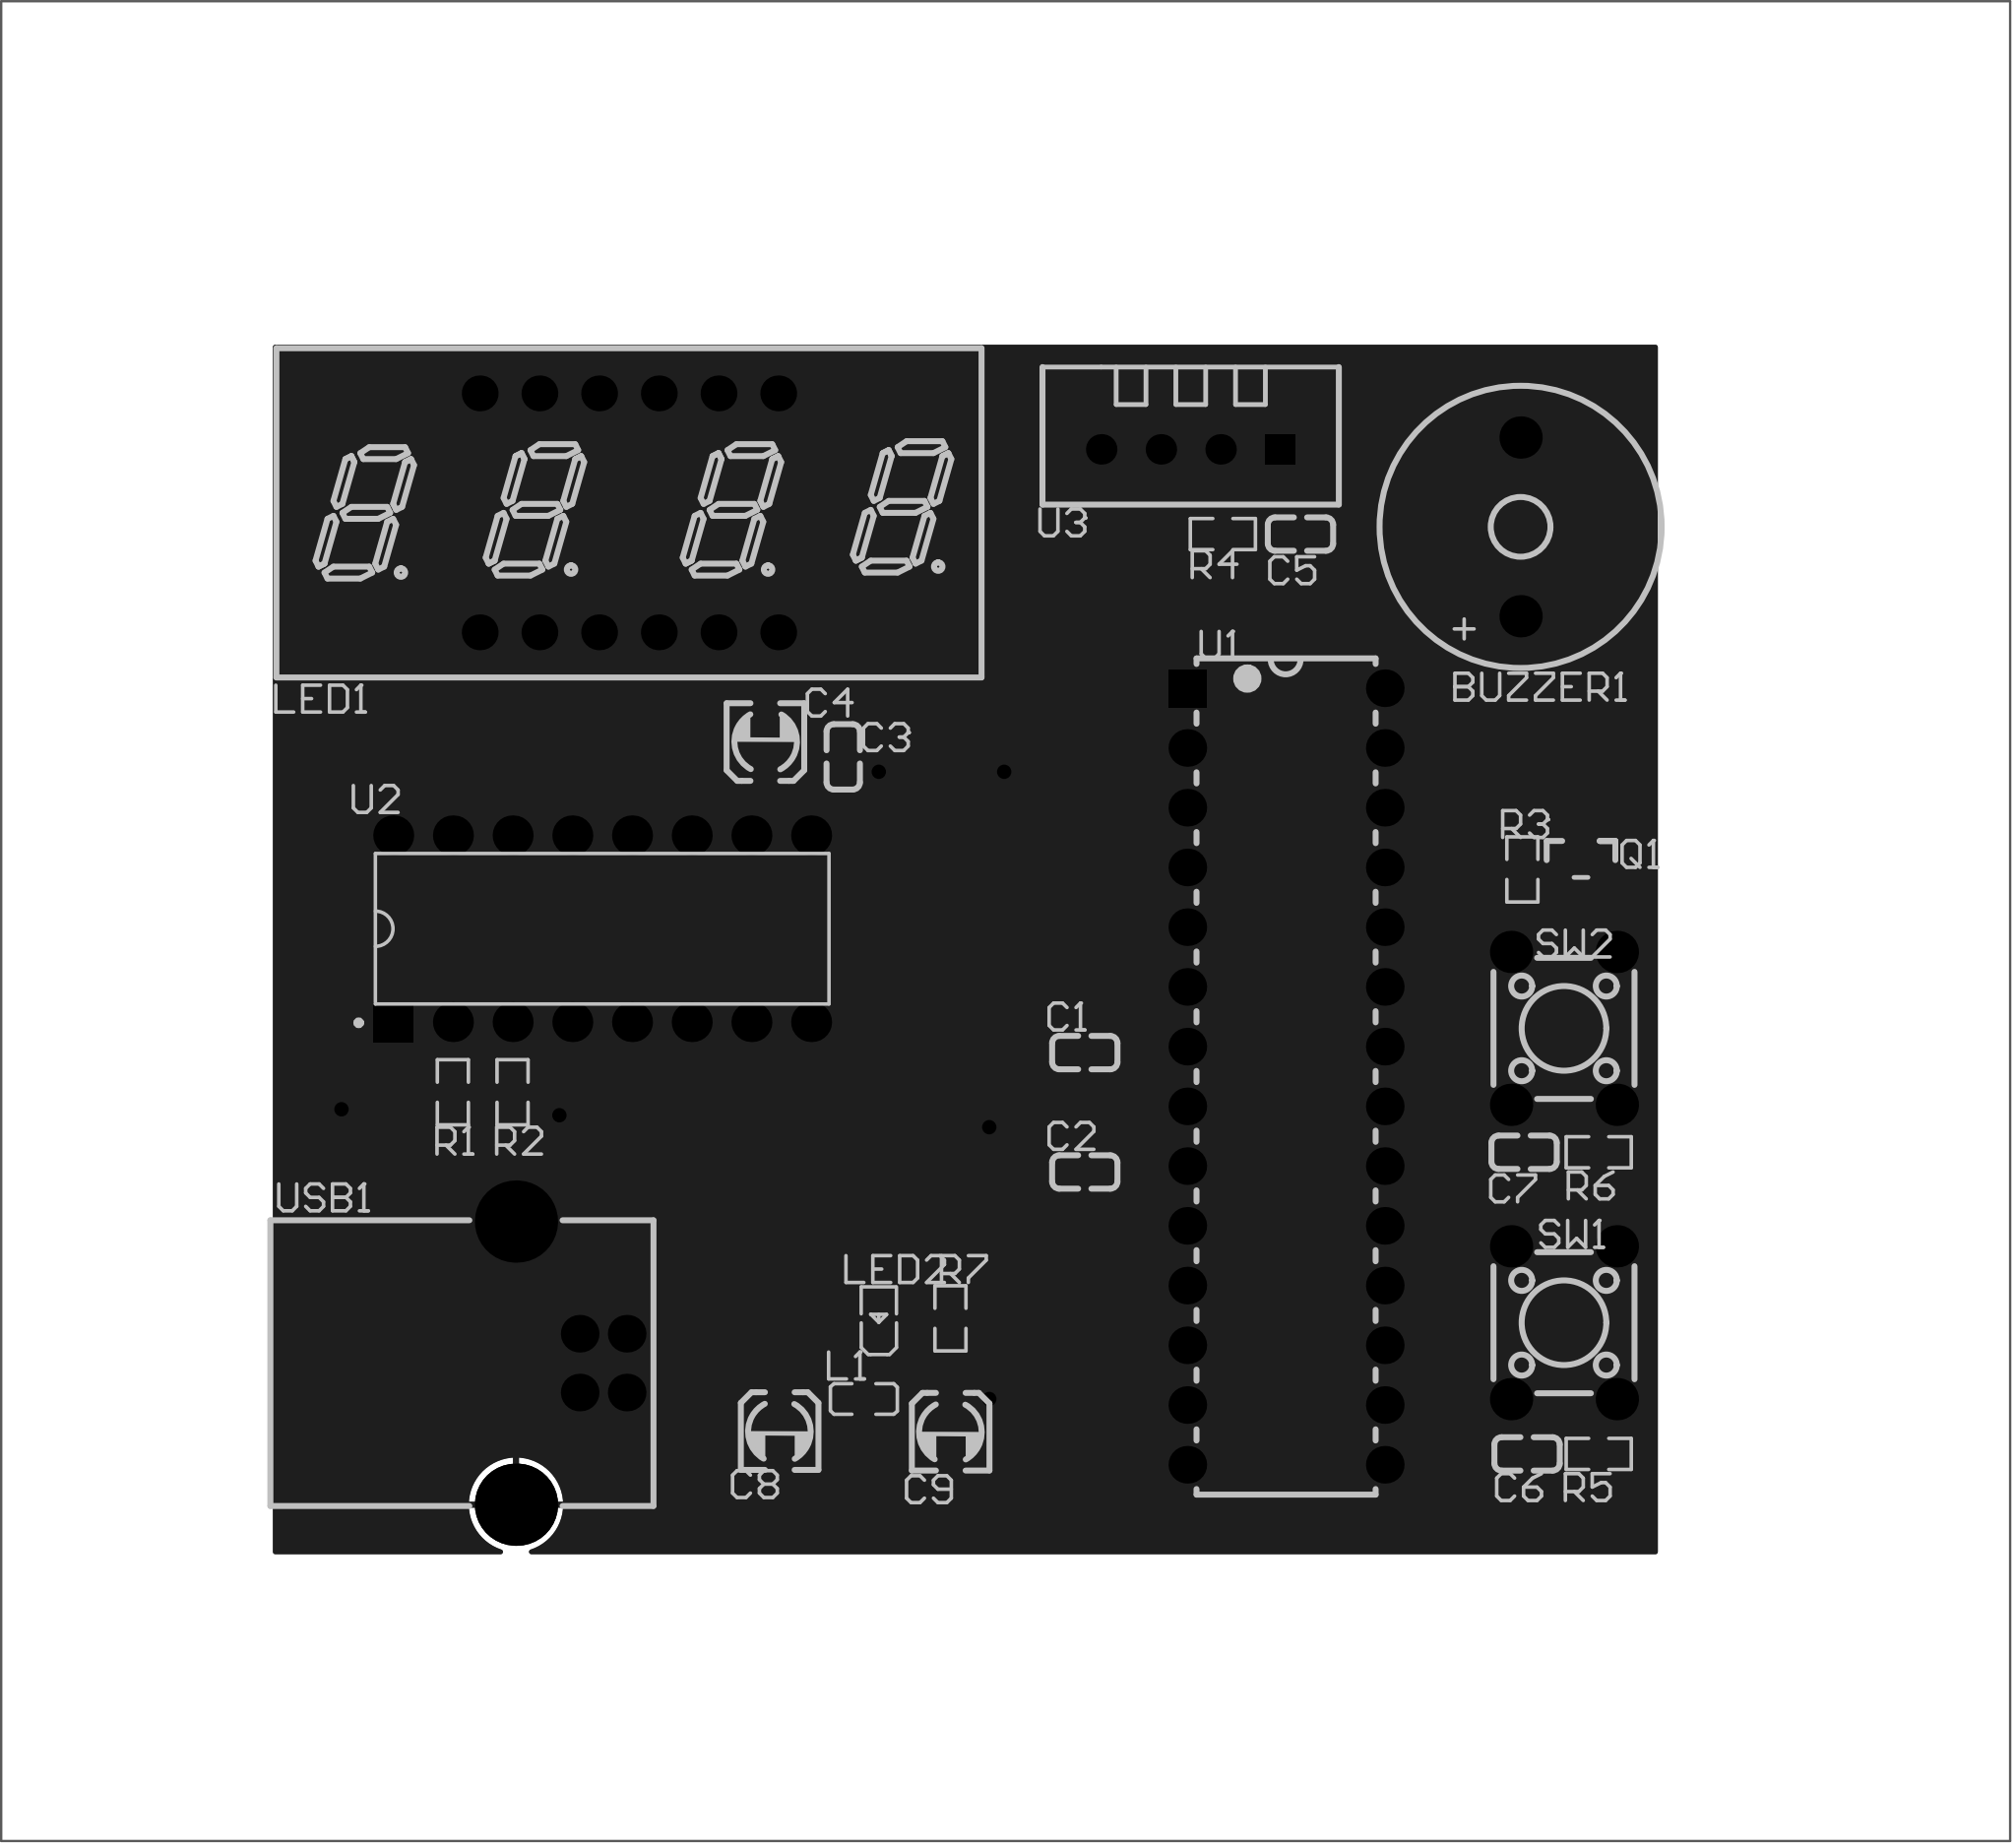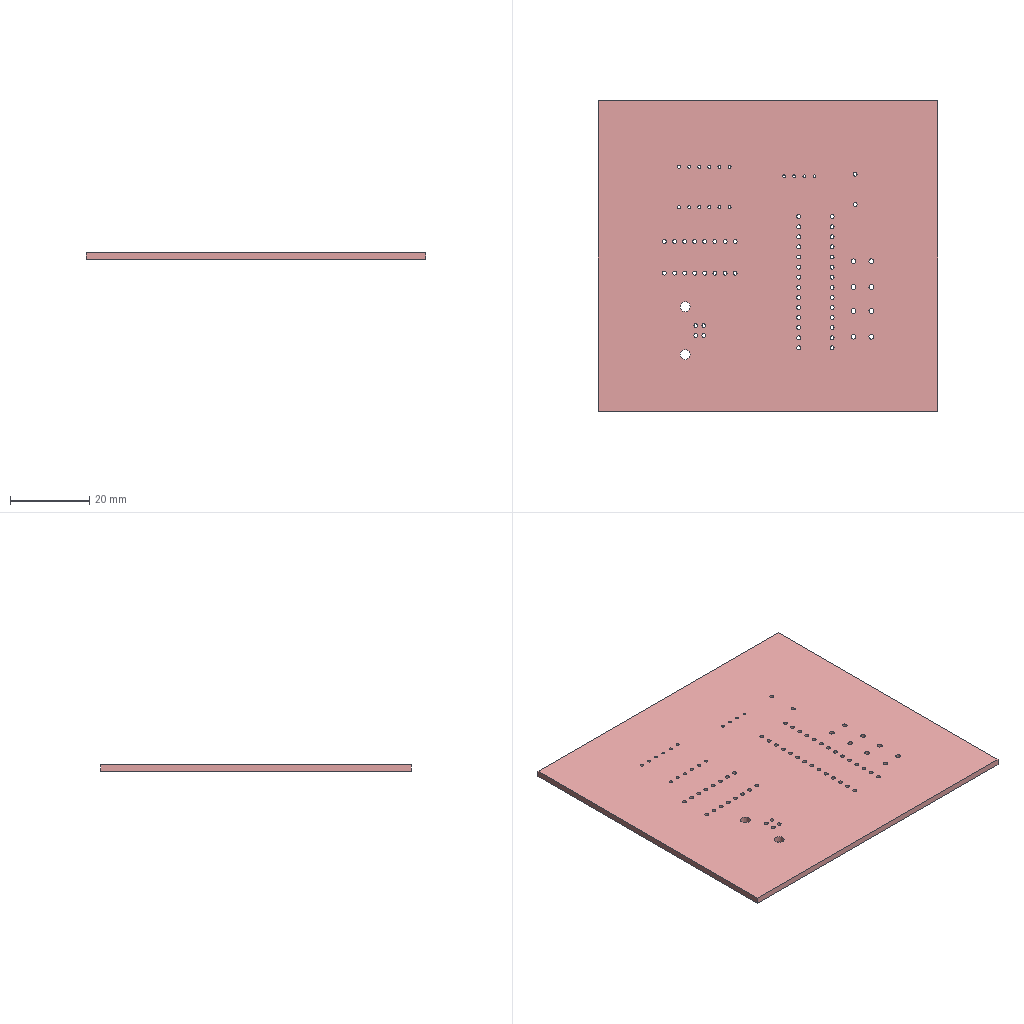Circuit board layout | Altium Designer | box 85.5 x 78.2 x 1.6 mm
Layer stack:
# Altium Designer layer stack of  (unit mm; dielectric type: 0 none, 1 core, 2 prepreg, 3 surface material)
index,name,kind,layer,copper_thickness_mm,dielectric_type,dielectric_thickness_mm,dielectric_material,dielectric_constant
0,Top Paste Mask Layer,other,,,,,,
1,Top Silkscreen Layer,other,,,,,,
2,Top Solder Mask Layer,dielectric,,,3,0.01,,3.3
3,Top Layer,copper,Top Layer,0.035,,,,
4,Dielectric1,dielectric,,,3,1.51,FR4,4.5
5,Bottom Layer,copper,Bottom Layer,0.035,,,,
6,Bottom Solder Mask Layer,dielectric,,,3,0.01,,3.3
7,Bottom Silkscreen Layer,other,,,,,,
8,Bottom Paste Mask Layer,other,,,,,,
# drill layer pairs: low layer,high layer
drill_pair,Top Layer,Bottom Layer
Part placement:
Designator,Comment,Layer,Footprint,Center-X(mm),Center-Y(mm),Rotation
BUZZER1,2.4kHz,TopLayer,BUZ-TH_BD12.0-P7.60-D0.6-FD,134.493,125.73,90
C1,1uF,TopLayer,C0603,115.952,103.374,0
C2,100nF,TopLayer,C0603,115.951,98.298,0
C3,100nF,TopLayer,C0603,105.675,115.95,270
C4,10uF,TopLayer,C_Ele_SMD_3x5.4mm,102.359,116.58,270
C5,100nF,TopLayer,C0603,125.128,125.424,180
C6,100nF,TopLayer,C0603,134.769,86.31,180
C7,100nF,TopLayer,C0603,134.642,99.137,180
C8,10uF,TopLayer,C_Ele_SMD_3x5.4mm,102.975,87.281,90
C9,10uF,TopLayer,C_Ele_SMD_3x5.4mm,110.25,87.254,90
L1,10uH,TopLayer,L0603,106.553,88.646,0
LED1,FJ3461AH,TopLayer,LED-SEG-TH_12P-L30.0-W14.0-P2.54-S10.16-BL,96.559,126.326,0
LED2,,TopLayer,LED_0603,107.196,92.024,90
Q1,,TopLayer,S8550P_SOT,137.063,111.724,270
R1,10K,TopLayer,R0603,89.066,101.688,270
R2,10K,TopLayer,R0603,91.606,101.688,270
R3,2K,TopLayer,R0603,134.569,111.163,270
R4,10K,TopLayer,R0603,121.826,125.424,0
R5,10K,TopLayer,R0603,137.817,86.31,180
R6,10K,TopLayer,R0603,137.817,99.137,180
R7,10K,TopLayer,R0603,110.236,92.075,270
SW1,,TopLayer,SW-TH_4P-L6.0-W6.0-P4.50-LS6.5,136.339,91.889,90
SW2,,TopLayer,SW-TH_4P-L6.0-W6.0-P4.50-LS6.5,136.339,104.405,90
U1,STC8H8K64U-45I-SKDIP28,TopLayer,DIP-28_L35.3-W7.3-P2.54-LS8.4-BL,124.515,102.358,270
U2,TM1650-DIP16,TopLayer,DIP-16_L19.3-W6.4-P2.54-LS8.0-BL,95.419,108.642,0
U3,DHT11,TopLayer,SENSOR-TH_DHT11,120.46,129.026,180
USB1,USB-B10-BRW,TopLayer,USB-B-TH_USB-B10-BRW,94.107,90.17,270
Pad and via stacks:
# Altium Designer via and pad stacks of  (unit mm). Each distinct definition once, with the count of objects using it.
# via: kind,start_layer,end_layer,hole_mm,diameter_mm,mode(0 simple;1 top-mid-bottom;2 full stack),diameter_per_layer,count,example_net
# pad: kind,layer,hole_mm,hole_type(0 round;1 square;2 slot),plating,top_size,top_shape(1 round;2 rect;3 octagon;9 rounded rect),mid_size,bottom_size,mode,footprint,size_per_layer,count,example
pad,Multi-Layer,1,0,plated,1.8x1.8,1,1.8x1.8,1.8x1.8,0,BUZ-TH_BD12.0-P7.60-D0.6-FD,,2,BUZZER1.2
pad,Multi-Layer,0.762,0,plated,1.524x1.524,1,1.524x1.524,1.524x1.524,0,LED-SEG-TH_12P-L30.0-W14.0-P2.54-S10.16-BL,,12,LED1.12
pad,Multi-Layer,1.2,0,plated,1.8x1.8,1,1.8x1.8,1.8x1.8,0,SW-TH_4P-L6.0-W6.0-P4.50-LS6.5,,8,SW1.1
pad,Multi-Layer,1,0,plated,1.6x1.6,1,1.6x1.6,1.6x1.6,0,DIP-28_L35.3-W7.3-P2.54-LS8.4-BL,,27,U1.26
pad,Multi-Layer,1,0,plated,1.6x1.6,2,1.6x1.6,1.6x1.6,0,DIP-28_L35.3-W7.3-P2.54-LS8.4-BL,,1,U1.1
pad,Multi-Layer,1,0,plated,1.7x1.7,2,1.7x1.7,1.7x1.7,0,DIP-16_L19.3-W6.4-P2.54-LS8.0-BL,,1,U2.1
pad,Multi-Layer,1,0,plated,1.7x1.7,1,1.7x1.7,1.7x1.7,0,DIP-16_L19.3-W6.4-P2.54-LS8.0-BL,,15,U2.2
pad,Multi-Layer,0.7112,0,plated,1.295x1.295,2,1.295x1.295,1.295x1.295,0,SENSOR-TH_DHT11,,1,U3.1
pad,Multi-Layer,0.7112,0,plated,1.295x1.295,1,1.295x1.295,1.295x1.295,0,SENSOR-TH_DHT11,,3,U3.2
pad,Multi-Layer,2.5,0,plated,3.5x3.5,1,3.5x3.5,3.5x3.5,0,USB-B-TH_USB-B10-BRW,,2,USB1.6
pad,Multi-Layer,1,0,plated,1.6x1.6,1,1.6x1.6,1.6x1.6,0,USB-B-TH_USB-B10-BRW,,4,USB1.4
pad,Top Layer,0,0,plated,0.8x0.9,2,0.8x0.9,0.8x0.9,0,C0603,,12,C1.2
pad,Top Layer,0,0,plated,1.999x0.8001,2,1.999x0.8001,1.999x0.8001,0,C_Ele_SMD_3x5.4mm,,6,C4.1
pad,Top Layer,0,0,plated,0.8x0.864,2,0.8x0.864,0.8x0.864,0,L0603,,2,L1.1
pad,Top Layer,0,0,plated,0.8001x0.8001,2,0.8001x0.8001,0.8001x0.8001,0,LED_0603,,2,LED2.1
pad,Top Layer,0,0,plated,0.701x1.25,2,0.701x1.25,0.701x1.25,0,S8550P_SOT,,3,Q1.3
pad,Top Layer,0,0,plated,0.8065x0.864,2,0.8065x0.864,0.8065x0.864,0,R0603,,14,R1.2
via,Top Layer,Bottom Layer,0.3048,0.61,0,,6,+5V
Copper pours:
name,layer,net,type(0 solid;1 hatched;2 none)
Top Layer-GND,Top Layer,GND,0
Bottom Layer-GND,Bottom Layer,GND,0